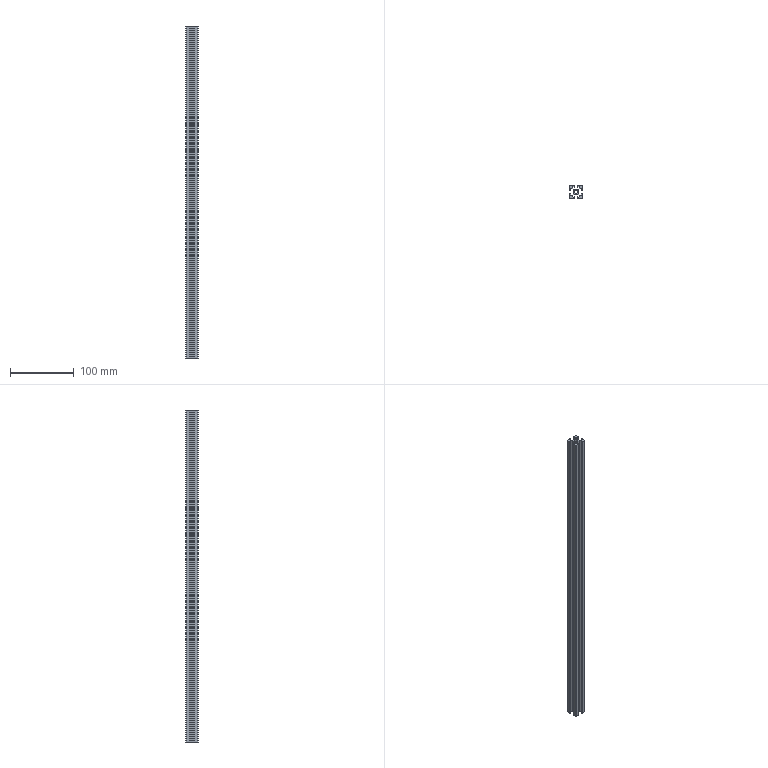Part | STEP file | AOB02-H2020_YHD013 | 1 solid | 80 faces | box 20 x 20 x 520 mm | volume 89774 mm3 | plane 74 | cylinder 6 | commonest cylinder face diameters 3 x4 5 x2